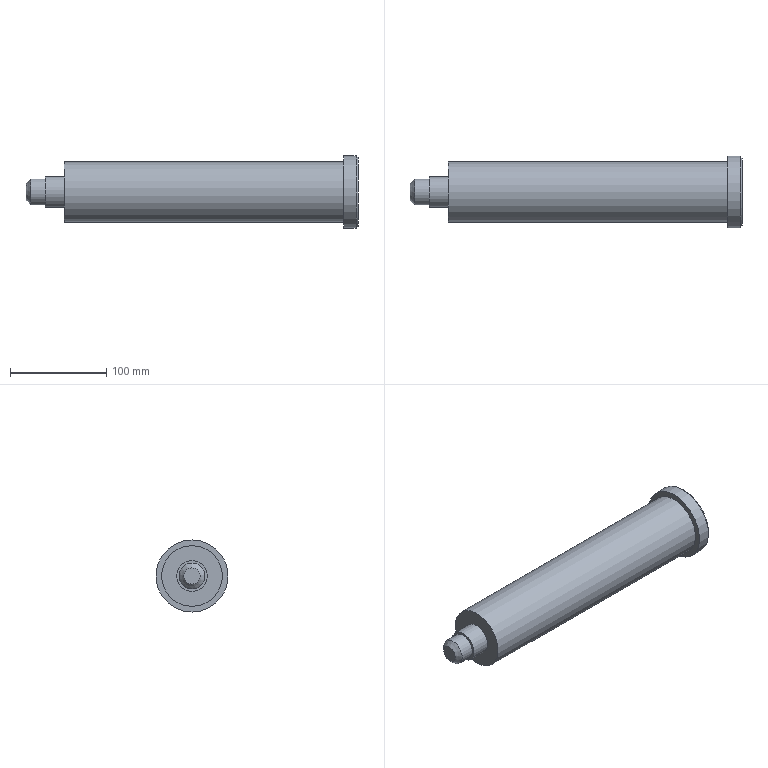Part | NX | features solid 2 | 1 solid | 11 faces | box 345 x 75 x 75 mm | volume 996413 mm3 | plane 5 | cylinder 4 | cone 2 | commonest cylinder face diameters 27 x1 32 x1 63 x1 75 x1
STEP:
#1=CARTESIAN_POINT('',(1124.,-715.,58.5));
#2=VERTEX_POINT('',#1);
#3=CARTESIAN_POINT('',(1124.,-715.,90.));
#4=DIRECTION('',(-1.,0.,0.));
#5=DIRECTION('',(0.,0.,-1.));
#6=AXIS2_PLACEMENT_3D('',#3,#4,#5);
#7=CIRCLE('',#6,31.5);
#8=EDGE_CURVE('',#2,#2,#7,.F.);
#9=ORIENTED_EDGE('',*,*,#8,.T.);
#10=EDGE_LOOP('',(#9));
#11=FACE_BOUND('',#10,.T.);
#12=CARTESIAN_POINT('',(1414.,-715.,121.5));
#13=VERTEX_POINT('',#12);
#14=CARTESIAN_POINT('',(1414.,-715.,90.));
#15=DIRECTION('',(1.,0.,0.));
#16=DIRECTION('',(0.,0.,1.));
#17=AXIS2_PLACEMENT_3D('',#14,#15,#16);
#18=CIRCLE('',#17,31.5);
#19=EDGE_CURVE('',#13,#13,#18,.T.);
#20=ORIENTED_EDGE('',*,*,#19,.F.);
#21=EDGE_LOOP('',(#20));
#22=FACE_BOUND('',#21,.T.);
#23=CARTESIAN_POINT('',(1104.,-715.,90.));
#24=DIRECTION('',(1.,0.,0.));
#25=DIRECTION('',(0.,0.,1.));
#26=AXIS2_PLACEMENT_3D('',#23,#24,#25);
#27=CYLINDRICAL_SURFACE('',#26,31.5);
#28=ADVANCED_FACE('',(#11,#22),#27,.T.);
#29=CARTESIAN_POINT('',(1124.,-715.,106.));
#30=VERTEX_POINT('',#29);
#31=CARTESIAN_POINT('',(1124.,-715.,90.));
#32=DIRECTION('',(1.,0.,0.));
#33=DIRECTION('',(0.,0.,1.));
#34=AXIS2_PLACEMENT_3D('',#31,#32,#33);
#35=CIRCLE('',#34,16.);
#36=EDGE_CURVE('',#30,#30,#35,.F.);
#37=ORIENTED_EDGE('',*,*,#36,.F.);
#38=EDGE_LOOP('',(#37));
#39=FACE_BOUND('',#38,.T.);
#40=ORIENTED_EDGE('',*,*,#8,.F.);
#41=EDGE_LOOP('',(#40));
#42=FACE_BOUND('',#41,.T.);
#43=CARTESIAN_POINT('',(1124.,-715.,90.));
#44=DIRECTION('',(1.,0.,0.));
#45=DIRECTION('',(0.,0.,1.));
#46=AXIS2_PLACEMENT_3D('',#43,#44,#45);
#47=PLANE('',#46);
#48=ADVANCED_FACE('',(#39,#42),#47,.F.);
#49=CARTESIAN_POINT('',(1427.,-715.,127.5));
#50=VERTEX_POINT('',#49);
#51=CARTESIAN_POINT('',(1427.,-715.,90.));
#52=DIRECTION('',(1.,0.,0.));
#53=DIRECTION('',(0.,0.,1.));
#54=AXIS2_PLACEMENT_3D('',#51,#52,#53);
#55=CIRCLE('',#54,37.5);
#56=EDGE_CURVE('',#50,#50,#55,.F.);
#57=ORIENTED_EDGE('',*,*,#56,.T.);
#58=EDGE_LOOP('',(#57));
#59=FACE_BOUND('',#58,.T.);
#60=CARTESIAN_POINT('',(1414.,-715.,127.5));
#61=VERTEX_POINT('',#60);
#62=CARTESIAN_POINT('',(1414.,-715.,90.));
#63=DIRECTION('',(1.,0.,0.));
#64=DIRECTION('',(0.,0.,1.));
#65=AXIS2_PLACEMENT_3D('',#62,#63,#64);
#66=CIRCLE('',#65,37.5);
#67=EDGE_CURVE('',#61,#61,#66,.T.);
#68=ORIENTED_EDGE('',*,*,#67,.T.);
#69=EDGE_LOOP('',(#68));
#70=FACE_BOUND('',#69,.T.);
#71=CARTESIAN_POINT('',(1414.,-715.,90.));
#72=DIRECTION('',(1.,0.,0.));
#73=DIRECTION('',(0.,0.,1.));
#74=AXIS2_PLACEMENT_3D('',#71,#72,#73);
#75=CYLINDRICAL_SURFACE('',#74,37.5);
#76=ADVANCED_FACE('',(#59,#70),#75,.T.);
#77=ORIENTED_EDGE('',*,*,#19,.T.);
#78=EDGE_LOOP('',(#77));
#79=FACE_BOUND('',#78,.T.);
#80=ORIENTED_EDGE('',*,*,#67,.F.);
#81=EDGE_LOOP('',(#80));
#82=FACE_BOUND('',#81,.T.);
#83=CARTESIAN_POINT('',(1414.,-715.,90.));
#84=DIRECTION('',(1.,0.,0.));
#85=DIRECTION('',(0.,0.,1.));
#86=AXIS2_PLACEMENT_3D('',#83,#84,#85);
#87=PLANE('',#86);
#88=ADVANCED_FACE('',(#79,#82),#87,.F.);
#89=CARTESIAN_POINT('',(1429.,-715.,125.5));
#90=VERTEX_POINT('',#89);
#91=CARTESIAN_POINT('',(1429.,-715.,90.));
#92=DIRECTION('',(1.,0.,0.));
#93=DIRECTION('',(0.,0.,1.));
#94=AXIS2_PLACEMENT_3D('',#91,#92,#93);
#95=CIRCLE('',#94,35.5);
#96=EDGE_CURVE('',#90,#90,#95,.T.);
#97=ORIENTED_EDGE('',*,*,#96,.T.);
#98=EDGE_LOOP('',(#97));
#99=FACE_BOUND('',#98,.T.);
#100=CARTESIAN_POINT('',(1429.,-715.,90.));
#101=DIRECTION('',(1.,0.,0.));
#102=DIRECTION('',(0.,0.,1.));
#103=AXIS2_PLACEMENT_3D('',#100,#101,#102);
#104=PLANE('',#103);
#105=ADVANCED_FACE('',(#99),#104,.T.);
#106=ORIENTED_EDGE('',*,*,#56,.F.);
#107=EDGE_LOOP('',(#106));
#108=FACE_BOUND('',#107,.T.);
#109=ORIENTED_EDGE('',*,*,#96,.F.);
#110=EDGE_LOOP('',(#109));
#111=FACE_BOUND('',#110,.T.);
#112=CARTESIAN_POINT('',(1429.,-715.,90.));
#113=DIRECTION('',(-1.,0.,0.));
#114=DIRECTION('',(0.,0.,-1.));
#115=AXIS2_PLACEMENT_3D('',#112,#113,#114);
#116=CONICAL_SURFACE('',#115,35.5,0.7854);
#117=ADVANCED_FACE('',(#108,#111),#116,.T.);
#118=CARTESIAN_POINT('',(1084.,-715.,98.5));
#119=VERTEX_POINT('',#118);
#120=CARTESIAN_POINT('',(1084.,-715.,90.));
#121=DIRECTION('',(1.,0.,0.));
#122=DIRECTION('',(0.,0.,1.));
#123=AXIS2_PLACEMENT_3D('',#120,#121,#122);
#124=CIRCLE('',#123,8.5);
#125=EDGE_CURVE('',#119,#119,#124,.F.);
#126=ORIENTED_EDGE('',*,*,#125,.T.);
#127=EDGE_LOOP('',(#126));
#128=FACE_BOUND('',#127,.T.);
#129=CARTESIAN_POINT('',(1084.,-715.,90.));
#130=DIRECTION('',(1.,0.,0.));
#131=DIRECTION('',(0.,0.,1.));
#132=AXIS2_PLACEMENT_3D('',#129,#130,#131);
#133=PLANE('',#132);
#134=ADVANCED_FACE('',(#128),#133,.F.);
#135=ORIENTED_EDGE('',*,*,#125,.F.);
#136=EDGE_LOOP('',(#135));
#137=FACE_BOUND('',#136,.T.);
#138=CARTESIAN_POINT('',(1089.,-715.,103.5));
#139=VERTEX_POINT('',#138);
#140=CARTESIAN_POINT('',(1089.,-715.,90.));
#141=DIRECTION('',(1.,0.,0.));
#142=DIRECTION('',(0.,0.,1.));
#143=AXIS2_PLACEMENT_3D('',#140,#141,#142);
#144=CIRCLE('',#143,13.5);
#145=EDGE_CURVE('',#139,#139,#144,.T.);
#146=ORIENTED_EDGE('',*,*,#145,.F.);
#147=EDGE_LOOP('',(#146));
#148=FACE_BOUND('',#147,.T.);
#149=CARTESIAN_POINT('',(1089.,-715.,90.));
#150=DIRECTION('',(1.,0.,0.));
#151=DIRECTION('',(0.,0.,1.));
#152=AXIS2_PLACEMENT_3D('',#149,#150,#151);
#153=CONICAL_SURFACE('',#152,13.5,0.7854);
#154=ADVANCED_FACE('',(#137,#148),#153,.T.);
#155=ORIENTED_EDGE('',*,*,#145,.T.);
#156=EDGE_LOOP('',(#155));
#157=FACE_BOUND('',#156,.T.);
#158=CARTESIAN_POINT('',(1104.,-715.,103.5));
#159=VERTEX_POINT('',#158);
#160=CARTESIAN_POINT('',(1104.,-715.,90.));
#161=DIRECTION('',(1.,0.,0.));
#162=DIRECTION('',(0.,0.,1.));
#163=AXIS2_PLACEMENT_3D('',#160,#161,#162);
#164=CIRCLE('',#163,13.5);
#165=EDGE_CURVE('',#159,#159,#164,.T.);
#166=ORIENTED_EDGE('',*,*,#165,.F.);
#167=EDGE_LOOP('',(#166));
#168=FACE_BOUND('',#167,.T.);
#169=CARTESIAN_POINT('',(1084.,-715.,90.));
#170=DIRECTION('',(1.,0.,0.));
#171=DIRECTION('',(0.,0.,1.));
#172=AXIS2_PLACEMENT_3D('',#169,#170,#171);
#173=CYLINDRICAL_SURFACE('',#172,13.5);
#174=ADVANCED_FACE('',(#157,#168),#173,.T.);
#175=ORIENTED_EDGE('',*,*,#165,.T.);
#176=EDGE_LOOP('',(#175));
#177=FACE_BOUND('',#176,.T.);
#178=CARTESIAN_POINT('',(1104.,-715.,106.));
#179=VERTEX_POINT('',#178);
#180=CARTESIAN_POINT('',(1104.,-715.,90.));
#181=DIRECTION('',(1.,0.,0.));
#182=DIRECTION('',(0.,0.,1.));
#183=AXIS2_PLACEMENT_3D('',#180,#181,#182);
#184=CIRCLE('',#183,16.);
#185=EDGE_CURVE('',#179,#179,#184,.T.);
#186=ORIENTED_EDGE('',*,*,#185,.F.);
#187=EDGE_LOOP('',(#186));
#188=FACE_BOUND('',#187,.T.);
#189=CARTESIAN_POINT('',(1104.,-715.,90.));
#190=DIRECTION('',(1.,0.,0.));
#191=DIRECTION('',(0.,0.,1.));
#192=AXIS2_PLACEMENT_3D('',#189,#190,#191);
#193=PLANE('',#192);
#194=ADVANCED_FACE('',(#177,#188),#193,.F.);
#195=ORIENTED_EDGE('',*,*,#185,.T.);
#196=EDGE_LOOP('',(#195));
#197=FACE_BOUND('',#196,.T.);
#198=ORIENTED_EDGE('',*,*,#36,.T.);
#199=EDGE_LOOP('',(#198));
#200=FACE_BOUND('',#199,.T.);
#201=CARTESIAN_POINT('',(1104.,-715.,90.));
#202=DIRECTION('',(1.,0.,0.));
#203=DIRECTION('',(0.,0.,1.));
#204=AXIS2_PLACEMENT_3D('',#201,#202,#203);
#205=CYLINDRICAL_SURFACE('',#204,16.);
#206=ADVANCED_FACE('',(#197,#200),#205,.T.);
#207=CLOSED_SHELL('',(#28,#48,#76,#88,#105,#117,#134,#154,#174,#194,#206));
#208=MANIFOLD_SOLID_BREP('',#207);
#209=(LENGTH_UNIT()NAMED_UNIT(*)SI_UNIT(.MILLI.,.METRE.));
#210=UNCERTAINTY_MEASURE_WITH_UNIT(LENGTH_MEASURE(0.00001),#209,'','');
#211=(NAMED_UNIT(*)PLANE_ANGLE_UNIT()SI_UNIT($,.RADIAN.));
#212=(NAMED_UNIT(*)SI_UNIT($,.STERADIAN.)SOLID_ANGLE_UNIT());
#213=(GEOMETRIC_REPRESENTATION_CONTEXT(3)GLOBAL_UNCERTAINTY_ASSIGNED_CONTEXT((#210))GLOBAL_UNIT_ASSIGNED_CONTEXT((#209,#211,#212))REPRESENTATION_CONTEXT('',''));
#214=ADVANCED_BREP_SHAPE_REPRESENTATION('',(#208),#213);